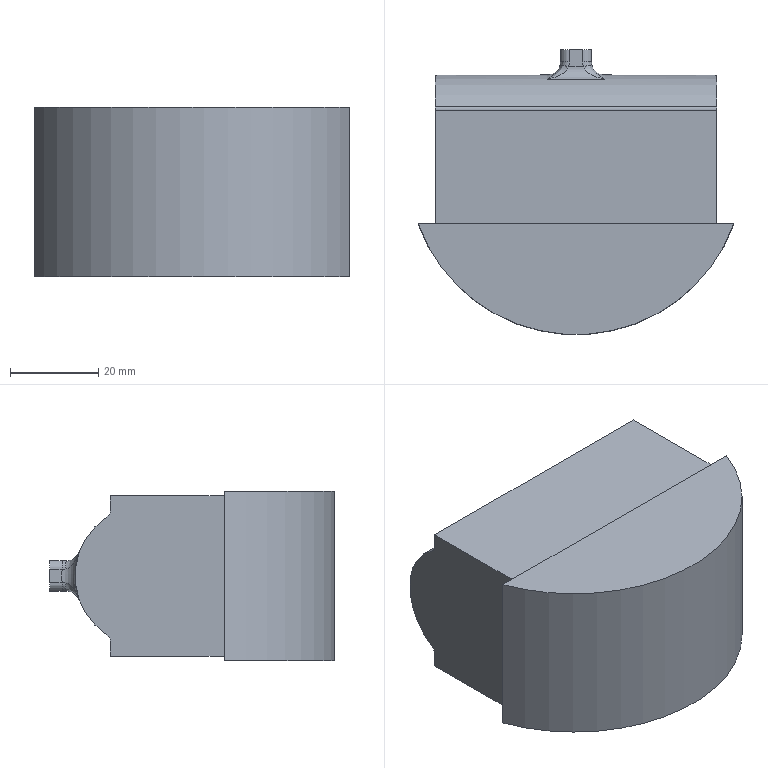NC program | NX | posted with a generic post | part box 71.627 x 64.667 x 38.42 mm
Lines 1 to 2470 of 24266, first 2159 of 2466 lines:
N10 G17 G21 G94 G90
(CAVITY_MILL , TOOL : D10)
N12 T00 M6
N14 G54
N16 G17 G0 G90 X23.164 Y-0.392 S2992 M3
N18 G43 Z10. H0
N20 Z0.2
N22 G94 G3 X14.3 Y0.708 Z-0.199 R-4.5 F1250.
N24 G1 Y-0.708 F2500.
N26 X14.41
N28 Y0.708
N30 X14.3
N32 Y5.208
N34 X8.926
N36 G2 X9.8 Y1.5 R8.3
N38 G1 Y-1.5
N40 G2 X8.926 Y-5.208 R8.3
N42 G1 X7.763 Y-4.627
N44 G2 X1.594 Y-8.499 R7.
N46 G1 X-1.599 Y-8.5
N48 G2 X-8.5 Y-1.5 R7.
N50 G1 Y1.5
N52 G2 X-1.5 Y8.5 R7.
N54 G1 X1.584
N56 G2 X8.5 Y1.5 R7.
N58 G1 Y-1.5
N60 G2 X7.763 Y-4.627 R7.
N62 G1 X8.926 Y-5.208
N64 X18.91
N66 Y5.208
N68 X14.3
N70 Y11.708
N72 X-14.3
N74 Y0.708
N76 X-14.41
N78 Y-0.708
N80 X-14.3
N82 Y0.708
N84 Y5.208
N86 X-18.91
N88 Y-5.208
N90 X-8.926
N92 G2 X-9.8 Y-1.5 R8.3
N94 G1 Y1.5
N96 G2 X-8.926 Y5.208 R8.3
N98 G1 X-14.3
N100 Y11.708
N102 X-25.41
N104 Y-11.708
N106 X25.41
N108 Y11.708
N110 X14.3
N112 Y18.208
N114 X-31.91
N116 Y-18.208
N118 X31.91
N120 Y18.208
N122 X14.3
N124 Y28.91
N126 Z0.001
N128 G0 Z0.3
N130 G1 X23.164 Y-0.392 F5000.
N132 G0 Z0.001
N134 G3 X14.3 Y0.708 Z-0.399 R-4.5 F1250.
N136 G1 Y-0.708 F2500.
N138 X14.41
N140 Y0.708
N142 X14.3
N144 Y5.208
N146 X8.926
N148 G2 X9.8 Y1.5 R8.3
N150 G1 Y-1.5
N152 G2 X8.926 Y-5.208 R8.3
N154 G1 X7.763 Y-4.627
N156 G2 X1.594 Y-8.499 R7.
N158 G1 X-1.599 Y-8.5
N160 G2 X-8.5 Y-1.5 R7.
N162 G1 Y1.5
N164 G2 X-1.5 Y8.5 R7.
N166 G1 X1.584
N168 G2 X8.5 Y1.5 R7.
N170 G1 Y-1.5
N172 G2 X7.763 Y-4.627 R7.
N174 G1 X8.926 Y-5.208
N176 X18.91
N178 Y5.208
N180 X14.3
N182 Y11.708
N184 X-14.3
N186 Y0.708
N188 X-14.41
N190 Y-0.708
N192 X-14.3
N194 Y0.708
N196 Y5.208
N198 X-18.91
N200 Y-5.208
N202 X-8.926
N204 G2 X-9.8 Y-1.5 R8.3
N206 G1 Y1.5
N208 G2 X-8.926 Y5.208 R8.3
N210 G1 X-14.3
N212 Y11.708
N214 X-25.41
N216 Y-11.708
N218 X25.41
N220 Y11.708
N222 X14.3
N224 Y18.208
N226 X-31.91
N228 Y-18.208
N230 X31.91
N232 Y18.208
N234 X14.3
N236 Y28.91
N238 Z-0.199
N240 G0 Z0.3
N242 G1 X23.164 Y-0.392 F5000.
N244 G0 Z-0.199
N246 G3 X14.3 Y0.708 Z-0.598 R-4.5 F1250.
N248 G1 Y-0.708 F2500.
N250 X14.41
N252 Y0.708
N254 X14.3
N256 Y5.208
N258 X8.926
N260 G2 X9.8 Y1.5 R8.3
N262 G1 Y-1.5
N264 G2 X8.926 Y-5.208 R8.3
N266 G1 X7.763 Y-4.627
N268 G2 X1.594 Y-8.499 R7.
N270 G1 X-1.599 Y-8.5
N272 G2 X-8.5 Y-1.5 R7.
N274 G1 Y1.5
N276 G2 X-1.5 Y8.5 R7.
N278 G1 X1.584
N280 G2 X8.5 Y1.5 R7.
N282 G1 Y-1.5
N284 G2 X7.763 Y-4.627 R7.
N286 G1 X8.926 Y-5.208
N288 X18.91
N290 Y5.208
N292 X14.3
N294 Y11.708
N296 X-14.3
N298 Y0.708
N300 X-14.41
N302 Y-0.708
N304 X-14.3
N306 Y0.708
N308 Y5.208
N310 X-18.91
N312 Y-5.208
N314 X-8.926
N316 G2 X-9.8 Y-1.5 R8.3
N318 G1 Y1.5
N320 G2 X-8.926 Y5.208 R8.3
N322 G1 X-14.3
N324 Y11.708
N326 X-25.41
N328 Y-11.708
N330 X25.41
N332 Y11.708
N334 X14.3
N336 Y18.208
N338 X-31.91
N340 Y-18.208
N342 X31.91
N344 Y18.208
N346 X14.3
N348 Y28.91
N350 Z-0.398
N352 G0 Z0.3
N354 G1 X23.164 Y-0.392 F5000.
N356 G0 Z-0.398
N358 G3 X14.3 Y0.708 Z-0.797 R-4.5 F1250.
N360 G1 Y-0.708 F2500.
N362 X14.41
N364 Y0.708
N366 X14.3
N368 Y5.208
N370 X8.926
N372 G2 X9.8 Y1.5 R8.3
N374 G1 Y-1.5
N376 G2 X8.926 Y-5.208 R8.3
N378 G1 X7.763 Y-4.627
N380 G2 X1.594 Y-8.499 R7.
N382 G1 X-1.599 Y-8.5
N384 G2 X-8.5 Y-1.5 R7.
N386 G1 Y1.5
N388 G2 X-1.5 Y8.5 R7.
N390 G1 X1.584
N392 G2 X8.5 Y1.5 R7.
N394 G1 Y-1.5
N396 G2 X7.763 Y-4.627 R7.
N398 G1 X8.926 Y-5.208
N400 X18.91
N402 Y5.208
N404 X14.3
N406 Y11.708
N408 X-14.3
N410 Y0.708
N412 X-14.41
N414 Y-0.708
N416 X-14.3
N418 Y0.708
N420 Y5.208
N422 X-18.91
N424 Y-5.208
N426 X-8.926
N428 G2 X-9.8 Y-1.5 R8.3
N430 G1 Y1.5
N432 G2 X-8.926 Y5.208 R8.3
N434 G1 X-14.3
N436 Y11.708
N438 X-25.41
N440 Y-11.708
N442 X25.41
N444 Y11.708
N446 X14.3
N448 Y18.208
N450 X-31.91
N452 Y-18.208
N454 X31.91
N456 Y18.208
N458 X14.3
N460 Y28.91
N462 Z-0.597
N464 G0 Z0.3
N466 G1 X23.164 Y-0.392 F5000.
N468 G0 Z-0.597
N470 G3 X14.3 Y0.708 Z-0.996 R-4.5 F1250.
N472 G1 Y-0.708 F2500.
N474 X14.41
N476 Y0.708
N478 X14.3
N480 Y5.208
N482 X8.926
N484 G2 X9.8 Y1.5 R8.3
N486 G1 Y-1.5
N488 G2 X8.926 Y-5.208 R8.3
N490 G1 X7.763 Y-4.627
N492 G2 X1.594 Y-8.499 R7.
N494 G1 X-1.599 Y-8.5
N496 G2 X-8.5 Y-1.5 R7.
N498 G1 Y1.5
N500 G2 X-1.5 Y8.5 R7.
N502 G1 X1.584
N504 G2 X8.5 Y1.5 R7.
N506 G1 Y-1.5
N508 G2 X7.763 Y-4.627 R7.
N510 G1 X8.926 Y-5.208
N512 X18.91
N514 Y5.208
N516 X14.3
N518 Y11.708
N520 X-14.3
N522 Y0.708
N524 X-14.41
N526 Y-0.708
N528 X-14.3
N530 Y0.708
N532 Y5.208
N534 X-18.91
N536 Y-5.208
N538 X-8.926
N540 G2 X-9.8 Y-1.5 R8.3
N542 G1 Y1.5
N544 G2 X-8.926 Y5.208 R8.3
N546 G1 X-14.3
N548 Y11.708
N550 X-25.41
N552 Y-11.708
N554 X25.41
N556 Y11.708
N558 X14.3
N560 Y18.208
N562 X-31.91
N564 Y-18.208
N566 X31.91
N568 Y18.208
N570 X14.3
N572 Y28.91
N574 Z-0.796
N576 G0 Z0.3
N578 G1 X23.164 Y-0.392 F5000.
N580 G0 Z-0.796
N582 G3 X14.3 Y0.708 Z-1.196 R-4.5 F1250.
N584 G1 Y-0.708 F2500.
N586 X14.41
N588 Y0.708
N590 X14.3
N592 Y5.208
N594 X8.926
N596 G2 X9.8 Y1.5 R8.3
N598 G1 Y-1.5
N600 G2 X8.926 Y-5.208 R8.3
N602 G1 X7.763 Y-4.627
N604 G2 X1.594 Y-8.499 R7.
N606 G1 X-1.599 Y-8.5
N608 G2 X-8.5 Y-1.5 R7.
N610 G1 Y1.5
N612 G2 X-1.5 Y8.5 R7.
N614 G1 X1.584
N616 G2 X8.5 Y1.5 R7.
N618 G1 Y-1.5
N620 G2 X7.763 Y-4.627 R7.
N622 G1 X8.926 Y-5.208
N624 X18.91
N626 Y5.208
N628 X14.3
N630 Y11.708
N632 X-14.3
N634 Y0.708
N636 X-14.41
N638 Y-0.708
N640 X-14.3
N642 Y0.708
N644 Y5.208
N646 X-18.91
N648 Y-5.208
N650 X-8.926
N652 G2 X-9.8 Y-1.5 R8.3
N654 G1 Y1.5
N656 G2 X-8.926 Y5.208 R8.3
N658 G1 X-14.3
N660 Y11.708
N662 X-25.41
N664 Y-11.708
N666 X25.41
N668 Y11.708
N670 X14.3
N672 Y18.208
N674 X-31.91
N676 Y-18.208
N678 X31.91
N680 Y18.208
N682 X14.3
N684 Y28.91
N686 Z-0.996
N688 G0 Z0.3
N690 G1 X23.164 Y-0.392 F5000.
N692 G0 Z-0.996
N694 G3 X14.3 Y0.708 Z-1.395 R-4.5 F1250.
N696 G1 Y-0.708 F2500.
N698 X14.41
N700 Y0.708
N702 X14.3
N704 Y5.208
N706 X8.926
N708 G2 X9.8 Y1.5 R8.3
N710 G1 Y-1.5
N712 G2 X8.926 Y-5.208 R8.3
N714 G1 X7.763 Y-4.627
N716 G2 X1.594 Y-8.499 R7.
N718 G1 X-1.599 Y-8.5
N720 G2 X-8.5 Y-1.5 R7.
N722 G1 Y1.5
N724 G2 X-1.5 Y8.5 R7.
N726 G1 X1.584
N728 G2 X8.5 Y1.5 R7.
N730 G1 Y-1.5
N732 G2 X7.763 Y-4.627 R7.
N734 G1 X8.926 Y-5.208
N736 X18.91
N738 Y5.208
N740 X14.3
N742 Y11.708
N744 X-14.3
N746 Y0.708
N748 X-14.41
N750 Y-0.708
N752 X-14.3
N754 Y0.708
N756 Y5.208
N758 X-18.91
N760 Y-5.208
N762 X-8.926
N764 G2 X-9.8 Y-1.5 R8.3
N766 G1 Y1.5
N768 G2 X-8.926 Y5.208 R8.3
N770 G1 X-14.3
N772 Y11.708
N774 X-25.41
N776 Y-11.708
N778 X25.41
N780 Y11.708
N782 X14.3
N784 Y18.208
N786 X-31.91
N788 Y-18.208
N790 X31.91
N792 Y18.208
N794 X14.3
N796 Y28.91
N798 Z-1.195
N800 G0 Z0.3
N802 G1 X23.164 Y-0.392 F5000.
N804 G0 Z-1.195
N806 G3 X14.3 Y0.708 Z-1.594 R-4.5 F1250.
N808 G1 Y-0.708 F2500.
N810 X14.41
N812 Y0.708
N814 X14.3
N816 Y5.208
N818 X8.926
N820 G2 X9.8 Y1.5 R8.3
N822 G1 Y-1.5
N824 G2 X8.926 Y-5.208 R8.3
N826 G1 X7.763 Y-4.627
N828 G2 X1.594 Y-8.499 R7.
N830 G1 X-1.599 Y-8.5
N832 G2 X-8.5 Y-1.5 R7.
N834 G1 Y1.5
N836 G2 X-1.5 Y8.5 R7.
N838 G1 X1.584
N840 G2 X8.5 Y1.5 R7.
N842 G1 Y-1.5
N844 G2 X7.763 Y-4.627 R7.
N846 G1 X8.926 Y-5.208
N848 X18.91
N850 Y5.208
N852 X14.3
N854 Y11.708
N856 X-14.3
N858 Y0.708
N860 X-14.41
N862 Y-0.708
N864 X-14.3
N866 Y0.708
N868 Y5.208
N870 X-18.91
N872 Y-5.208
N874 X-8.926
N876 G2 X-9.8 Y-1.5 R8.3
N878 G1 Y1.5
N880 G2 X-8.926 Y5.208 R8.3
N882 G1 X-14.3
N884 Y11.708
N886 X-25.41
N888 Y-11.708
N890 X25.41
N892 Y11.708
N894 X14.3
N896 Y18.208
N898 X-31.91
N900 Y-18.208
N902 X31.91
N904 Y18.208
N906 X14.3
N908 Y28.91
N910 Z-1.394
N912 G0 Z0.3
N914 G1 X23.164 Y-0.392 F5000.
N916 G0 Z-1.394
N918 G3 X14.3 Y0.708 Z-1.793 R-4.5 F1250.
N920 G1 Y-0.708 F2500.
N922 X14.41
N924 Y0.708
N926 X14.3
N928 Y5.208
N930 X8.926
N932 G2 X9.8 Y1.5 R8.3
N934 G1 Y-1.5
N936 G2 X8.926 Y-5.208 R8.3
N938 G1 X7.763 Y-4.627
N940 G2 X1.594 Y-8.499 R7.
N942 G1 X-1.599 Y-8.5
N944 G2 X-8.5 Y-1.5 R7.
N946 G1 Y1.5
N948 G2 X-1.5 Y8.5 R7.
N950 G1 X1.584
N952 G2 X8.5 Y1.5 R7.
N954 G1 Y-1.5
N956 G2 X7.763 Y-4.627 R7.
N958 G1 X8.926 Y-5.208
N960 X18.91
N962 Y5.208
N964 X14.3
N966 Y11.708
N968 X-14.3
N970 Y0.708
N972 X-14.41
N974 Y-0.708
N976 X-14.3
N978 Y0.708
N980 Y5.208
N982 X-18.91
N984 Y-5.208
N986 X-8.926
N988 G2 X-9.8 Y-1.5 R8.3
N990 G1 Y1.5
N992 G2 X-8.926 Y5.208 R8.3
N994 G1 X-14.3
N996 Y11.708
N998 X-25.41
N1000 Y-11.708
N1002 X25.41
N1004 Y11.708
N1006 X14.3
N1008 Y18.208
N1010 X-31.91
N1012 Y-18.208
N1014 X31.91
N1016 Y18.208
N1018 X14.3
N1020 Y28.91
N1022 Z-1.593
N1024 G0 Z0.3
N1026 G1 X23.164 Y-0.392 F5000.
N1028 G0 Z-1.593
N1030 G3 X14.3 Y0.708 Z-1.993 R-4.5 F1250.
N1032 G1 Y-0.708 F2500.
N1034 X14.41
N1036 Y0.708
N1038 X14.3
N1040 Y5.208
N1042 X8.926
N1044 G2 X9.8 Y1.5 R8.3
N1046 G1 Y-1.5
N1048 G2 X8.926 Y-5.208 R8.3
N1050 G1 X7.763 Y-4.627
N1052 G2 X1.594 Y-8.499 R7.
N1054 G1 X-1.599 Y-8.5
N1056 G2 X-8.5 Y-1.5 R7.
N1058 G1 Y1.5
N1060 G2 X-1.5 Y8.5 R7.
N1062 G1 X1.584
N1064 G2 X8.5 Y1.5 R7.
N1066 G1 Y-1.5
N1068 G2 X7.763 Y-4.627 R7.
N1070 G1 X8.926 Y-5.208
N1072 X18.91
N1074 Y5.208
N1076 X14.3
N1078 Y11.708
N1080 X-14.3
N1082 Y0.708
N1084 X-14.41
N1086 Y-0.708
N1088 X-14.3
N1090 Y0.708
N1092 Y5.208
N1094 X-18.91
N1096 Y-5.208
N1098 X-8.926
N1100 G2 X-9.8 Y-1.5 R8.3
N1102 G1 Y1.5
N1104 G2 X-8.926 Y5.208 R8.3
N1106 G1 X-14.3
N1108 Y11.708
N1110 X-25.41
N1112 Y-11.708
N1114 X25.41
N1116 Y11.708
N1118 X14.3
N1120 Y18.208
N1122 X-31.91
N1124 Y-18.208
N1126 X31.91
N1128 Y18.208
N1130 X14.3
N1132 Y28.91
N1134 Z-1.793
N1136 G0 Z0.3
N1138 G1 X23.164 Y-0.392 F5000.
N1140 G0 Z-1.793
N1142 G3 X14.3 Y0.708 Z-2.192 R-4.5 F1250.
N1144 G1 Y-0.708 F2500.
N1146 X14.41
N1148 Y0.708
N1150 X14.3
N1152 Y5.208
N1154 X8.926
N1156 G2 X9.8 Y1.5 R8.3
N1158 G1 Y-1.5
N1160 G2 X8.926 Y-5.208 R8.3
N1162 G1 X7.763 Y-4.627
N1164 G2 X1.594 Y-8.499 R7.
N1166 G1 X-1.599 Y-8.5
N1168 G2 X-8.5 Y-1.5 R7.
N1170 G1 Y1.5
N1172 G2 X-1.5 Y8.5 R7.
N1174 G1 X1.584
N1176 G2 X8.5 Y1.5 R7.
N1178 G1 Y-1.5
N1180 G2 X7.763 Y-4.627 R7.
N1182 G1 X8.926 Y-5.208
N1184 X18.91
N1186 Y5.208
N1188 X14.3
N1190 Y11.708
N1192 X-14.3
N1194 Y0.708
N1196 X-14.41
N1198 Y-0.708
N1200 X-14.3
N1202 Y0.708
N1204 Y5.208
N1206 X-18.91
N1208 Y-5.208
N1210 X-8.926
N1212 G2 X-9.8 Y-1.5 R8.3
N1214 G1 Y1.5
N1216 G2 X-8.926 Y5.208 R8.3
N1218 G1 X-14.3
N1220 Y11.708
N1222 X-25.41
N1224 Y-11.708
N1226 X25.41
N1228 Y11.708
N1230 X14.3
N1232 Y18.208
N1234 X-31.91
N1236 Y-18.208
N1238 X31.91
N1240 Y18.208
N1242 X14.3
N1244 Y28.91
N1246 Z-1.992
N1248 G0 Z0.3
N1250 G1 X23.164 Y-0.392 F5000.
N1252 G0 Z-1.992
N1254 G3 X14.3 Y0.708 Z-2.391 R-4.5 F1250.
N1256 G1 Y-0.708 F2500.
N1258 X14.41
N1260 Y0.708
N1262 X14.3
N1264 Y5.208
N1266 X8.926
N1268 G2 X9.8 Y1.5 R8.3
N1270 G1 Y-1.5
N1272 G2 X8.926 Y-5.208 R8.3
N1274 G1 X7.763 Y-4.627
N1276 G2 X1.594 Y-8.499 R7.
N1278 G1 X-1.599 Y-8.5
N1280 G2 X-8.5 Y-1.5 R7.
N1282 G1 Y1.5
N1284 G2 X-1.5 Y8.5 R7.
N1286 G1 X1.584
N1288 G2 X8.5 Y1.5 R7.
N1290 G1 Y-1.5
N1292 G2 X7.763 Y-4.627 R7.
N1294 G1 X8.926 Y-5.208
N1296 X18.91
N1298 Y5.208
N1300 X14.3
N1302 Y11.708
N1304 X-14.3
N1306 Y0.708
N1308 X-14.41
N1310 Y-0.708
N1312 X-14.3
N1314 Y0.708
N1316 Y5.208
N1318 X-18.91
N1320 Y-5.208
N1322 X-8.926
N1324 G2 X-9.8 Y-1.5 R8.3
N1326 G1 Y1.5
N1328 G2 X-8.926 Y5.208 R8.3
N1330 G1 X-14.3
N1332 Y11.708
N1334 X-25.41
N1336 Y-11.708
N1338 X25.41
N1340 Y11.708
N1342 X14.3
N1344 Y18.208
N1346 X-31.91
N1348 Y-18.208
N1350 X31.91
N1352 Y18.208
N1354 X14.3
N1356 Y28.91
N1358 Z-2.191
N1360 G0 Z0.3
N1362 G1 X23.164 Y-0.392 F5000.
N1364 G0 Z-2.191
N1366 G3 X14.3 Y0.708 Z-2.591 R-4.5 F1250.
N1368 G1 Y-0.708 F2500.
N1370 X14.41
N1372 Y0.708
N1374 X14.3
N1376 Y5.208
N1378 X8.926
N1380 G2 X9.8 Y1.5 R8.3
N1382 G1 Y-1.5
N1384 G2 X8.926 Y-5.208 R8.3
N1386 G1 X7.763 Y-4.627
N1388 G2 X1.594 Y-8.499 R7.
N1390 G1 X-1.599 Y-8.5
N1392 G2 X-8.5 Y-1.5 R7.
N1394 G1 Y1.5
N1396 G2 X-1.5 Y8.5 R7.
N1398 G1 X1.584
N1400 G2 X8.5 Y1.5 R7.
N1402 G1 Y-1.5
N1404 G2 X7.763 Y-4.627 R7.
N1406 G1 X8.926 Y-5.208
N1408 X18.91
N1410 Y5.208
N1412 X14.3
N1414 Y11.708
N1416 X-14.3
N1418 Y0.708
N1420 X-14.41
N1422 Y-0.708
N1424 X-14.3
N1426 Y0.708
N1428 Y5.208
N1430 X-18.91
N1432 Y-5.208
N1434 X-8.926
N1436 G2 X-9.8 Y-1.5 R8.3
N1438 G1 Y1.5
N1440 G2 X-8.926 Y5.208 R8.3
N1442 G1 X-14.3
N1444 Y11.708
N1446 X-25.41
N1448 Y-11.708
N1450 X25.41
N1452 Y11.708
N1454 X14.3
N1456 Y18.208
N1458 X-31.91
N1460 Y-18.208
N1462 X31.91
N1464 Y18.208
N1466 X14.3
N1468 Y28.91
N1470 Z-2.391
N1472 G0 Z0.3
N1474 G1 X23.164 Y-0.392 F5000.
N1476 G0 Z-2.391
N1478 G3 X14.3 Y0.708 Z-2.79 R-4.5 F1250.
N1480 G1 Y-0.708 F2500.
N1482 X14.41
N1484 Y0.708
N1486 X14.3
N1488 Y5.208
N1490 X8.926
N1492 G2 X9.8 Y1.5 R8.3
N1494 G1 Y-1.5
N1496 G2 X8.926 Y-5.208 R8.3
N1498 G1 X7.763 Y-4.627
N1500 G2 X1.594 Y-8.499 R7.
N1502 G1 X-1.599 Y-8.5
N1504 G2 X-8.5 Y-1.5 R7.
N1506 G1 Y1.5
N1508 G2 X-1.5 Y8.5 R7.
N1510 G1 X1.584
N1512 G2 X8.5 Y1.5 R7.
N1514 G1 Y-1.5
N1516 G2 X7.763 Y-4.627 R7.
N1518 G1 X8.926 Y-5.208
N1520 X18.91
N1522 Y5.208
N1524 X14.3
N1526 Y11.708
N1528 X-14.3
N1530 Y0.708
N1532 X-14.41
N1534 Y-0.708
N1536 X-14.3
N1538 Y0.708
N1540 Y5.208
N1542 X-18.91
N1544 Y-5.208
N1546 X-8.926
N1548 G2 X-9.8 Y-1.5 R8.3
N1550 G1 Y1.5
N1552 G2 X-8.926 Y5.208 R8.3
N1554 G1 X-14.3
N1556 Y11.708
N1558 X-25.41
N1560 Y-11.708
N1562 X25.41
N1564 Y11.708
N1566 X14.3
N1568 Y18.208
N1570 X-31.91
N1572 Y-18.208
N1574 X31.91
N1576 Y18.208
N1578 X14.3
N1580 Y28.91
N1582 Z-2.59
N1584 G0 Z0.3
N1586 G1 X23.184 Y-0.376 F5000.
N1588 G0 Z-2.59
N1590 G3 X14.318 Y0.708 Z-2.989 R-4.5 F1250.
N1592 G1 X14.321 Y-0.708 F2500.
N1594 X14.41
N1596 Y0.708
N1598 X14.318
N1600 Y5.208
N1602 X8.938
N1604 G2 X9.79 Y1.997 R8.239
N1606 G1 X9.815 Y1.577
N1608 X9.817 Y1.503
N1610 X9.822 Y-1.498
N1612 X9.819 Y-1.592
N1614 X9.79 Y-2.006
N1616 G2 X8.935 Y-5.208 R8.288
N1618 G1 X7.771 Y-4.628
N1620 G2 X1.858 Y-8.491 R6.988
N1622 X1.594 Y-8.499 R7.
N1624 G1 X-1.599 Y-8.5
N1626 G2 X-1.886 Y-8.489 R7.
N1628 X-8.517 Y-1.5 R7.012
N1630 G1 X-8.522 Y1.5
N1632 X-8.496 Y1.922
N1634 G2 X-1.939 Y8.486 R6.994
N1636 X-1.5 Y8.5 R7.
N1638 G1 X1.584
N1640 G2 X4.913 Y7.612 R7.
N1642 X8.492 Y1.922 R6.939
N1644 G1 X8.517 Y1.5
N1646 X8.522 Y-1.5
N1648 X8.492 Y-1.922
N1650 G2 X7.771 Y-4.628 R6.988
N1652 G1 X8.935 Y-5.208
N1654 X18.91
N1656 Y5.208
N1658 X14.318
N1660 Y11.708
N1662 X-14.321
N1664 Y0.708
N1666 X-14.41
N1668 Y-0.708
N1670 X-14.318
N1672 X-14.321 Y0.708
N1674 Y5.208
N1676 X-18.91
N1678 Y-5.208
N1680 X-8.938
N1682 G2 X-9.817 Y-1.503 R8.312
N1684 G1 X-9.822 Y1.498
N1686 X-9.82 Y1.582
N1688 X-9.793 Y2.002
N1690 G2 X-8.936 Y5.208 R8.294
N1692 G1 X-14.321
N1694 Y11.708
N1696 X-25.41
N1698 Y-11.708
N1700 X25.41
N1702 Y11.708
N1704 X14.318
N1706 Y18.208
N1708 X-31.91
N1710 Y-18.208
N1712 X31.91
N1714 Y18.208
N1716 X14.318
N1718 Y28.91
N1720 Z-2.789
N1722 G0 Z0.3
N1724 G1 X23.211 Y-0.382 F5000.
N1726 G0 Z-2.789
N1728 G3 X14.346 Y0.708 Z-3.188 R-4.5 F1250.
N1730 G1 X14.348 Y-0.708 F2500.
N1732 X14.41
N1734 Y0.708
N1736 X14.346
N1738 Y5.208
N1740 X8.963
N1742 G2 X9.81 Y2.008 R8.182
N1744 G1 X9.841 Y1.602
N1746 X9.845 Y1.502
N1748 X9.849 Y-1.499
N1750 X9.844 Y-1.613
N1752 X9.809 Y-2.017
N1754 G2 X8.955 Y-5.208 R8.282
N1756 G1 X7.792 Y-4.628
N1758 G2 X1.88 Y-8.49 R6.982
N1760 X1.594 Y-8.499 R7.
N1762 G1 X-1.599 Y-8.5
N1764 G2 X-1.877 Y-8.49 R7.
N1766 X-8.517 Y-1.922 R6.992
N1768 G1 X-8.545 Y-1.501
N1770 X-8.549 Y1.501
N1772 X-8.514 Y1.922
N1774 G2 X-1.909 Y8.488 R6.984
N1776 X-1.587 Y8.499 R7.
N1778 G1 X1.584 Y8.5
N1780 G2 X4.913 Y7.612 R7.
N1782 X8.512 Y1.922 R6.882
N1784 G1 X8.545 Y1.501
N1786 X8.549 Y-1.501
N1788 X8.512 Y-1.922
N1790 G2 X7.792 Y-4.628 R6.982
N1792 G1 X8.955 Y-5.208
N1794 X18.91
N1796 Y5.208
N1798 X14.346
N1800 Y11.708
N1802 X-14.348
N1804 Y0.708
N1806 X-14.41
N1808 Y-0.708
N1810 X-14.346
N1812 X-14.348 Y0.708
N1814 Y5.208
N1816 X-18.91
N1818 Y-5.208
N1820 X-8.958
N1822 G2 X-9.815 Y-2.004 R8.292
N1824 G1 X-9.842 Y-1.587
N1826 X-9.845 Y-1.502
N1828 X-9.849 Y1.499
N1830 X-9.844 Y1.606
N1832 X-9.811 Y2.014
N1834 G2 X-8.957 Y5.208 R8.284
N1836 G1 X-14.348
N1838 Y11.708
N1840 X-25.41
N1842 Y-11.708
N1844 X25.41
N1846 Y11.708
N1848 X14.346
N1850 Y18.208
N1852 X-31.91
N1854 Y-18.208
N1856 X31.91
N1858 Y18.208
N1860 X14.346
N1862 Y28.91
N1864 Z-2.988
N1866 G0 Z0.3
N1868 G1 X23.238 Y-0.388 F5000.
N1870 G0 Z-2.988
N1872 G3 X14.374 Y0.708 Z-3.388 R-4.5 F1250.
N1874 G1 X14.375 Y-0.708 F2500.
N1876 X14.41
N1878 Y0.708
N1880 X14.374
N1882 Y5.208
N1884 X8.983
N1886 G2 X9.84 Y2.008 R8.288
N1888 G1 X9.87 Y1.595
N1890 X9.874 Y1.502
N1892 X9.875 Y-1.501
N1894 X9.871 Y-1.605
N1896 X9.838 Y-2.013
N1898 G2 X8.982 Y-5.208 R8.29
N1900 G1 X7.819 Y-4.627
N1902 G2 X1.858 Y-8.491 R6.99
N1904 X1.594 Y-8.499 R7.
N1906 G1 X-1.599 Y-8.5
N1908 G2 X-1.877 Y-8.49 R7.
N1910 X-8.543 Y-1.922 R6.995
N1912 G1 X-8.574 Y-1.501
N1914 X-8.575 Y1.501
N1916 X-8.541 Y1.922
N1918 G2 X-1.909 Y8.488 R6.989
N1920 X-1.587 Y8.499 R7.
N1922 G1 X1.584 Y8.5
N1924 G2 X2.099 Y8.474 R7.
N1926 X8.543 Y1.922 R6.988
N1928 G1 X8.574 Y1.501
N1930 X8.575 Y-1.501
N1932 X8.541 Y-1.922
N1934 G2 X7.819 Y-4.627 R6.99
N1936 G1 X8.982 Y-5.208
N1938 X18.91
N1940 Y5.208
N1942 X14.374
N1944 Y11.708
N1946 X-14.375
N1948 Y0.708
N1950 X-14.41
N1952 Y-0.708
N1954 X-14.374
N1956 X-14.375 Y0.708
N1958 Y5.208
N1960 X-18.91
N1962 Y-5.208
N1964 X-8.982
N1966 G2 X-9.84 Y-2.009 R8.295
N1968 G1 X-9.87 Y-1.595
N1970 X-9.874 Y-1.502
N1972 X-9.875 Y1.501
N1974 X-9.871 Y1.605
N1976 X-9.838 Y2.013
N1978 G2 X-8.982 Y5.208 R8.289
N1980 G1 X-14.375
N1982 Y11.708
N1984 X-25.41
N1986 Y-11.708
N1988 X25.41
N1990 Y11.708
N1992 X14.374
N1994 Y18.208
N1996 X-31.91
N1998 Y-18.208
N2000 X31.91
N2002 Y18.208
N2004 X14.374
N2006 Y28.91
N2008 Z-3.188
N2010 G0 Z0.3
N2012 G1 X17.435 Y8.208 F5000.
N2014 G0 Z-3.188
N2016 G3 X9.023 Y5.208 Z-3.587 R-4.5 F1250.
N2018 G2 X9.911 Y1.525 R8.327 F2500.
N2020 G1 X9.92 Y1.191
N2022 X9.921 Y1.153
N2024 Y-1.153
N2026 X9.92 Y-1.191
N2028 X9.911 Y-1.525
N2030 G2 X9.023 Y-5.208 R8.332
N2032 G1 X7.861 Y-4.623
N2034 G2 X1.858 Y-8.491 R7.032
N2036 X1.594 Y-8.499 R7.
N2038 G1 X-1.599 Y-8.5
N2040 G2 X-1.877 Y-8.49 R7.
N2042 X-8.611 Y-1.502 R7.029
N2044 G1 X-8.621 Y-1.153
N2046 Y1.153
N2048 X-8.611 Y1.502
N2050 G2 X-1.909 Y8.488 R7.027
N2052 X-1.587 Y8.499 R7.
N2054 G1 X1.584 Y8.5
N2056 G2 X2.099 Y8.474 R7.
N2058 X8.611 Y1.502 R7.027
N2060 G1 X8.621 Y1.153
N2062 Y-1.153
N2064 X8.611 Y-1.502
N2066 G2 X7.861 Y-4.623 R7.032
N2068 G1 X9.023 Y-5.208
N2070 X18.91
N2072 Y5.208
N2074 X9.023
N2076 Y11.708
N2078 X-9.024
N2080 Y5.208
N2082 X-18.91
N2084 Y-5.208
N2086 X-9.023
N2088 G2 X-9.911 Y-1.524 R8.329
N2090 G1 X-9.92 Y-1.191
N2092 X-9.921 Y-1.153
N2094 Y1.153
N2096 X-9.92 Y1.191
N2098 X-9.911 Y1.524
N2100 G2 X-9.024 Y5.208 R8.327
N2102 G1 Y11.708
N2104 X-25.41
N2106 Y-11.708
N2108 X25.41
N2110 Y11.708
N2112 X9.023
N2114 Y18.208
N2116 X-31.91
N2118 Y-18.208
N2120 X31.91
N2122 Y18.208
N2124 X9.023
N2126 Y28.91
N2128 Z-3.387
N2130 G0 Z0.3
N2132 G1 X17.5 Y8.202 F5000.
N2134 G0 Z-3.387
N2136 G3 X9.085 Y5.208 Z-3.786 R-4.5 F1250.
N2138 G2 X9.968 Y1.547 R8.308 F2500.
N2140 G1 X9.98 Y1.198
N2142 X9.981 Y1.153
N2144 Y-1.153
N2146 X9.98 Y-1.197
N2148 X9.968 Y-1.546
N2150 G2 X9.085 Y-5.208 R8.318
N2152 G1 X7.921 Y-4.624
N2154 G2 X1.858 Y-8.491 R7.018
N2156 X1.594 Y-8.499 R7.
N2158 G1 X-1.599 Y-8.5
N2160 G2 X-1.877 Y-8.49 R7.
N2162 X-8.576 Y-2.691 R7.063
N2164 X-8.576 Y2.691 R28.187
N2166 X-1.909 Y8.488 R7.057
N2168 X-1.587 Y8.499 R7.
N2170 G1 X1.584 Y8.5
N2172 G2 X2.099 Y8.474 R7.
N2174 X8.652 Y1.922 R7.008
N2176 G1 X8.669 Y1.503
N2178 X8.681 Y1.153
N2180 Y-1.153
N2182 X8.669 Y-1.503
N2184 X8.653 Y-1.922
N2186 G2 X7.921 Y-4.624 R7.018
N2188 G1 X9.085 Y-5.208
N2190 X18.91
N2192 Y5.208
N2194 X9.085
N2196 Y11.708
N2198 X-9.089
N2200 Y5.208
N2202 X-18.91
N2204 Y-5.208
N2206 X-9.088
N2208 G2 X-9.855 Y-2.923 R8.363
N2210 G1 X-9.87 Y-2.815
N2212 G2 X-9.87 Y2.815 R29.488
N2214 G1 X-9.855 Y2.922
N2216 G2 X-9.089 Y5.208 R8.357
N2218 G1 Y11.708
N2220 X-25.41
N2222 Y-11.708
N2224 X25.41
N2226 Y11.708
N2228 X9.085
N2230 Y18.208
N2232 X-31.91
N2234 Y-18.208
N2236 X31.91
N2238 Y18.208
N2240 X9.085
N2242 Y28.91
N2244 Z-3.586
N2246 G0 Z0.3
N2248 G1 X17.592 Y8.186 F5000.
N2250 G0 Z-3.586
N2252 G3 X9.171 Y5.208 Z-3.986 R-4.5 F1250.
N2254 G2 X10.035 Y1.932 R8.306 F2500.
N2256 X10.038 Y-1.989 R37.796
N2258 X9.182 Y-5.208 R8.22
N2260 G1 X8.019 Y-4.626
N2262 G2 X4.621 Y-7.861 R6.92
N2264 G1 X4.351 Y-7.974
N2266 G2 X1.714 Y-8.501 R6.854
N2268 G1 X1.42
N2270 Y-8.5
N2272 X-1.372
N2274 Y-8.501
N2276 X-1.584
N2278 Y-8.5
N2280 X-1.599
N2282 X-1.657 Y-8.498
N2284 G2 X-8.737 Y-1.922 R7.008
N2286 G1 X-8.754 Y-1.504
N2288 G2 X-8.74 Y1.922 R36.496
N2290 X-4.621 Y7.861 R6.92
N2292 X-1.679 Y8.498 R6.882
N2294 G1 X-1.61 Y8.499
N2296 Y8.501
N2298 X-1.372
N2300 Y8.5
N2302 X1.42
N2304 Y8.501
N2306 X1.741
N2308 G2 X8.737 Y1.864 R7.006
N2310 X8.74 Y-1.922 R36.496
N2312 X8.019 Y-4.626 R6.92
N2314 G1 X9.182 Y-5.208
N2316 X18.91
N2318 Y5.208
N2320 X9.171
N2322 Y11.708
N2324 X-9.182
N2326 Y5.208
N2328 X-18.91
N2330 Y-5.208
N2332 X-9.176
N2334 G2 X-10.053 Y-1.559 R8.308
N2336 X-10.038 Y1.989 R37.796
N2338 X-9.182 Y5.208 R8.22
N2340 G1 Y11.708
N2342 X-25.41
N2344 Y-11.708
N2346 X25.41
N2348 Y11.708
N2350 X9.171
N2352 Y18.208
N2354 X-31.91
N2356 Y-18.208
N2358 X31.91
N2360 Y18.208
N2362 X9.171
N2364 Y28.91
N2366 Z-3.786
N2368 G0 Z0.3
N2370 G1 X17.734 Y8.157 F5000.
N2372 G0 Z-3.786
N2374 G3 X9.303 Y5.208 Z-4.185 R-4.5 F1250.
N2376 G2 X10.133 Y1.981 R8.054 F2500.
N2378 X10.133 Y-1.982 R41.78
N2380 X9.303 Y-5.208 R8.141
N2382 G1 X8.137 Y-4.633
N2384 G2 X4.621 Y-7.927 R6.841
N2386 G1 X4.447 Y-7.998
N2388 G2 X1.8 Y-8.514 R7.045
N2390 G1 X-1.658
N2392 G2 X-6.751 Y-6.536 R7.262
N2394 X-8.834 Y-1.922 R6.833
N2396 X-8.834 Y1.937 R40.464
N2398 X-5.006 Y7.74 R6.815
N2400 G1 X-4.861 Y7.811
N2402 G2 X-1.807 Y8.514 R6.984
N2404 G1 X1.672
N2406 G2 X7.942 Y4.998 R7.088
N2408 X8.834 Y1.922 R6.754
N2410 X8.834 Y-1.922 R40.48
N2412 X8.137 Y-4.633 R6.841
N2414 G1 X9.303 Y-5.208
N2416 X18.91
N2418 Y5.208
N2420 X9.303
N2422 Y11.708
N2424 X-9.301
N2426 Y5.208
N2428 X-18.91
N2430 Y-5.208
N2432 X-9.305
N2434 G2 X-10.133 Y-1.982 R8.133
N2436 X-10.132 Y2. R41.764
N2438 X-9.301 Y5.208 R8.115
N2440 G1 Y11.708
N2442 X-25.41
N2444 Y-11.708
N2446 X25.41
N2448 Y11.708
N2450 X9.303
N2452 Y18.208
N2454 X-31.91
N2456 Y-18.208
N2458 X31.91
N2460 Y18.208
N2462 X9.303
N2464 Y28.91
N2466 Z-3.985
N2468 G0 Z0.3
N2470 G1 X17.914 Y8.036 F5000.
N2472 G0 Z-3.985
N2474 G3 X9.442 Y5.208 Z-4.384 R-4.5 F1250.
N2476 G2 X10.245 Y1.984 R8.3 F2500.
N2478 X10.245 Y-1.981 R37.26
N2480 X9.443 Y-5.208 R8.115
N2482 G1 X8.272 Y-4.642
N2484 G2 X3.851 Y-8.272 R6.815
N2486 X1.831 Y-8.54 R6.997
N2488 G1 X-1.785
N2490 G2 X-7.603 Y-5.767 R7.192
N2492 X-8.947 Y-1.922 R7.031
N2494 X-8.947 Y1.922 R35.931
N2496 X-3.851 Y8.272 R6.815
N2498 X-1.895 Y8.54 R6.893
N2500 G1 X1.804
N2502 G2 X7.6 Y5.767 R7.19
N2504 X8.947 Y1.922 R7.
N2506 X8.947 Y-1.922 R35.96
N2508 X8.272 Y-4.642 R6.815
N2510 G1 X9.443 Y-5.208
N2512 X18.91
N2514 Y5.208
N2516 X9.442
N2518 Y11.708
N2520 X-9.443
N2522 Y5.208
N2524 X-18.91
N2526 Y-5.208
N2528 X-9.443
N2530 G2 X-10.245 Y-1.985 R8.331
N2532 X-10.245 Y1.981 R37.231
N2534 X-9.443 Y5.208 R8.115
N2536 G1 Y11.708
N2538 X-25.41
N2540 Y-11.708
N2542 X25.41
N2544 Y11.708
N2546 X9.442
N2548 Y18.208
N2550 X-31.91
N2552 Y-18.208
N2554 X31.91
N2556 Y18.208
N2558 X9.442
N2560 Y28.91
N2562 Z-4.184
N2564 G0 Z0.3
N2566 G1 X18.126 Y7.911 F5000.
N2568 G0 Z-4.184
N2570 G3 X9.613 Y5.208 Z-4.583 R-4.5 F1250.
N2572 G2 X10.282 Y2.849 R7.967 F2500.
N2574 X10.306 Y-2.677 R26.083
N2576 X9.609 Y-5.208 R7.908
N2578 G1 X8.431 Y-4.659
N2580 G2 X5.011 Y-7.96 R6.608
N2582 G1 X4.741 Y-8.074
N2584 G2 X2.06 Y-8.58 R7.047
N2586 G1 X-2.06
N2588 G2 X-7.147 Y-6.536 R7.282
N2590 X-8.992 Y-2.691 R6.667
N2592 X-9.011 Y2.559 R24.783
N2594 X-5.02 Y7.956 R6.59
N2596 G1 X-4.741 Y8.074
N2598 G2 X-1.964 Y8.58 R7.193
N2600 G1 X2.06
N2602 G2 X7.147 Y6.536 R7.267
N2604 X8.992 Y2.691 R6.667
N2606 X9.013 Y-2.545 R24.783
N2608 X8.431 Y-4.659 R6.608
N2610 G1 X9.609 Y-5.208
N2612 X18.91
N2614 Y5.208
N2616 X9.613
N2618 Y11.708
N2620 X-9.612
N2622 Y5.208
N2624 X-18.91
N2626 Y-5.208
N2628 X-9.613
N2630 G2 X-10.282 Y-2.849 R7.967
N2632 X-10.304 Y2.692 R26.083
N2634 X-9.612 Y5.208 R7.89
N2636 G1 Y11.708
N2638 X-25.41
N2640 Y-11.708
N2642 X25.41
N2644 Y11.708
N2646 X9.613
N2648 Y18.208
N2650 X-31.91
N2652 Y-18.208
N2654 X31.91
N2656 Y18.208
N2658 X9.613
N2660 Y28.91
N2662 Z-4.383
N2664 G0 Z0.3
N2666 G1 X18.351 Y7.804 F5000.
N2668 G0 Z-4.383
N2670 G3 X9.805 Y5.208 Z-4.783 R-4.5 F1250.
N2672 G2 X10.442 Y2.84 R7.923 F2500.
N2674 X10.445 Y-2.841 R23.274
N2676 X9.801 Y-5.208 R7.901
N2678 G1 X8.614 Y-4.675
N2680 G2 X3.851 Y-8.453 R6.601
N2682 X2.252 Y-8.634 R6.14
N2684 G1 X-2.252
N2686 G2 X-6.162 Y-7.535 R7.46
N2688 X-9.151 Y-2.691 R6.541
N2690 X-9.133 Y2.851 R21.868
N2692 X-4.197 Y8.368 R6.559
N2694 G1 X-3.851 Y8.453
N2696 G2 X-2.252 Y8.634 R7.951
N2698 G1 X2.108
N2700 G2 X6.932 Y6.969 R7.311
N2702 X9.151 Y2.691 R6.623
N2704 X9.154 Y-2.691 R21.974
N2706 X8.614 Y-4.675 R6.601
N2708 G1 X9.801 Y-5.208
N2710 X18.91
N2712 Y5.208
N2714 X9.805
N2716 Y11.708
N2718 X-9.804
N2720 Y5.208
N2722 X-18.91
N2724 Y-5.208
N2726 X-9.808
N2728 G2 X-10.442 Y-2.839 R7.841
N2730 X-10.422 Y3.019 R23.168
N2732 X-9.804 Y5.208 R7.859
N2734 G1 Y11.708
N2736 X-25.41
N2738 Y-11.708
N2740 X25.41
N2742 Y11.708
N2744 X9.805
N2746 Y18.208
N2748 X-31.91
N2750 Y-18.208
N2752 X31.91
N2754 Y18.208
N2756 X9.805
N2758 Y28.91
N2760 Z-4.583
N2762 G0 Z0.3
N2764 G1 X18.641 Y7.61 F5000.
N2766 G0 Z-4.583
N2768 G3 X10.038 Y5.208 Z-4.982 R-4.5 F1250.
N2770 G2 X10.469 Y3.784 R7.321 F2500.
N2772 X10.524 Y-3.476 R19.751
N2774 X10.021 Y-5.208 R7.695
N2776 G1 X8.824 Y-4.701
N2778 G2 X5.392 Y-8.115 R6.395
N2780 X2.311 Y-8.703 R7.439
N2782 G1 X-2.472
N2784 G2 X-9.013 Y-4.229 R6.752
N2786 X-9.013 Y4.229 R17.194
N2788 X-3.081 Y8.682 R6.693
N2790 G1 X-2.311 Y8.703
N2792 X2.59
N2794 G2 X7.645 Y6.536 R6.977
N2796 X9.193 Y3.536 R6.021
N2798 X9.243 Y-3.255 R18.451
N2800 X8.824 Y-4.701 R6.395
N2802 G1 X10.021 Y-5.208
N2804 X18.91
N2806 Y5.208
N2808 X10.038
N2810 Y11.708
N2812 X-10.023
N2814 Y5.208
N2816 X-18.91
N2818 Y-5.208
N2820 X-10.021
N2822 G2 X-10.237 Y-4.667 R8.052
N2824 G1 X-10.273 Y-4.549
N2826 G2 X-10.273 Y4.549 R18.494
N2828 G1 X-10.239 Y4.662
N2830 G2 X-10.023 Y5.208 R7.993
N2832 G1 Y11.708
N2834 X-25.41
N2836 Y-11.708
N2838 X25.41
N2840 Y11.708
N2842 X10.038
N2844 Y18.208
N2846 X-31.91
N2848 Y-18.208
N2850 X31.91
N2852 Y18.208
N2854 X10.038
N2856 Y28.91
N2858 Z-4.782
N2860 G0 Z0.3
N2862 G1 X18.915 Y7.474 F5000.
N2864 G0 Z-4.782
N2866 G3 X10.276 Y5.208 Z-5.181 R-4.5 F1250.
N2868 G2 X10.642 Y4.013 R7.563 F2500.
N2870 X10.705 Y-3.704 R18.835
N2872 X10.271 Y-5.208 R7.699
N2874 G1 X9.065 Y-4.722
N2876 G2 X4.57 Y-8.565 R6.399
N2878 X2.609 Y-8.789 R8.713
N2880 G1 X-2.973
N2882 G2 X-9.388 Y-3.62 R6.565
N2884 X-9.241 Y4.229 R16.991
N2886 X-3.081 Y8.783 R6.562
N2888 G1 X-2.723 Y8.789
N2890 X2.859
N2892 G2 X6.826 Y7.546 R6.953
N2894 X9.372 Y3.736 R6.263
N2896 X9.428 Y-3.46 R17.535
N2898 X9.065 Y-4.722 R6.399
N2900 G1 X10.271 Y-5.208
N2902 X18.91
N2904 Y5.208
N2906 X10.276
N2908 Y11.708
N2910 X-10.264
N2912 Y5.208
N2914 X-18.91
N2916 Y-5.208
N2918 X-10.25
N2920 G2 X-10.658 Y-3.897 R7.865
N2922 X-10.5 Y4.553 R18.291
N2924 X-10.264 Y5.208 R7.862
N2926 G1 Y11.708
N2928 X-25.41
N2930 Y-11.708
N2932 X25.41
N2934 Y11.708
N2936 X10.276
N2938 Y18.208
N2940 X-31.91
N2942 Y-18.208
N2944 X31.91
N2946 Y18.208
N2948 X10.276
N2950 Y28.91
N2952 Z-4.981
N2954 G0 Z0.3
N2956 G1 X19.219 Y7.292 F5000.
N2958 G0 Z-4.981
N2960 G3 X10.534 Y5.208 Z-5.38 R-4.5 F1250.
N2962 G2 X10.737 Y4.585 R7.612 F2500.
N2964 X10.942 Y-3.758 R16.425
N2966 G1 X10.825 Y-4.258
N2968 G2 X10.536 Y-5.208 R7.625
N2970 G1 X9.32 Y-4.749
N2972 G2 X4.467 Y-8.755 R6.325
N2974 X2.847 Y-8.893 R9.605
N2976 G1 X-2.908
N2978 G2 X-4.595 Y-8.732 R8.964
N2980 X-9.487 Y-4.229 R6.312
N2982 X-9.677 Y3.46 R15.125
N2984 G1 X-9.562 Y3.95
N2986 G2 X-3.864 Y8.846 R6.368
N2988 X-2.694 Y8.893 R14.827
N2990 G1 X2.897
N2992 G2 X4.571 Y8.737 R9.077
N2994 X9.487 Y4.229 R6.312
N2996 X9.677 Y-3.46 R15.125
N2998 G1 X9.559 Y-3.962
N3000 G2 X9.32 Y-4.749 R6.325
N3002 G1 X10.536 Y-5.208
N3004 X18.91
N3006 Y5.208
N3008 X10.534
N3010 Y11.708
N3012 X-10.535
N3014 Y5.208
N3016 X-18.91
N3018 Y-5.208
N3020 X-10.534
N3022 G2 X-10.737 Y-4.585 R7.612
N3024 X-10.942 Y3.758 R16.425
N3026 G1 X-10.828 Y4.246
N3028 G2 X-10.535 Y5.208 R7.668
N3030 G1 Y11.708
N3032 X-25.41
N3034 Y-11.708
N3036 X25.41
N3038 Y11.708
N3040 X10.534
N3042 Y18.208
N3044 X-31.91
N3046 Y-18.208
N3048 X31.91
N3050 Y18.208
N3052 X10.534
N3054 Y28.91
N3056 Z-5.18
N3058 G0 Z0.3
N3060 G1 X19.613 Y6.917 F5000.
N3062 G0 Z-5.18
N3064 G3 X10.847 Y5.208 Z-5.58 R-4.5 F1250.
N3066 G1 X11.031 Y4.644 F2500.
N3068 G2 X10.843 Y-5.208 R14.289
N3070 G1 X9.631 Y-4.736
N3072 G2 X9.178 Y-5.767 R12.989
N3074 X3.851 Y-9.012 R6.497
N3076 G1 X3.32 Y-9.017
N3078 X-3.081
N3080 X-3.141 Y-9.019
N3082 G2 X-9.548 Y-4.998 R6.538
N3084 G1 X-9.799 Y-4.229
N3086 G2 X-9.178 Y5.767 R12.989
N3088 X-3.851 Y9.012 R6.482
N3090 G1 X-3.32 Y9.017
N3092 X3.081
N3094 X3.141 Y9.019
N3096 G2 X9.548 Y4.998 R6.538
N3098 G1 X9.799 Y4.229
N3100 G2 X9.631 Y-4.736 R12.989
N3102 G1 X10.843 Y-5.208
N3104 X18.91
N3106 Y5.208
N3108 X10.847
N3110 Y11.708
N3112 X-10.843
N3114 Y5.208
N3116 X-18.91
N3118 Y-5.208
N3120 X-10.847
N3122 X-11.031 Y-4.644
N3124 G2 X-10.843 Y5.208 R14.289
N3126 G1 Y11.708
N3128 X-25.41
N3130 Y-11.708
N3132 X25.41
N3134 Y11.708
N3136 X10.847
N3138 Y18.208
N3140 X-31.91
N3142 Y-18.208
N3144 X31.91
N3146 Y18.208
N3148 X10.847
N3150 Y28.91
N3152 Z-5.38
N3154 G0 Z0.3
N3156 G1 X4.832 Y-14.807 F5000.
N3158 G0 Z-5.38
N3160 G3 X-4.032 Y-13.708 Z-5.779 R-4.5 F1250.
N3162 G1 X0.468
N3164 X27.41 F2500.
N3166 Y-10.463
N3168 X11.612
N3170 G2 X3.928 Y-13.664 R10.82
N3172 G1 X-3.9
N3174 G2 X-11.619 Y-10.463 R10.906
N3176 G1 X-27.41
N3178 Y-13.708
N3180 X0.468
N3182 Y-18.208
N3184 X31.91
N3186 Y-5.963
N3188 X9.425
N3190 G2 X3.928 Y-9.164 R6.32
N3192 G1 X-3.9
N3194 G2 X-9.447 Y-5.963 R6.406
N3196 G1 X-31.91
N3198 Y-18.208
N3200 X0.468
N3202 Y-28.91
N3204 Z-5.579
N3206 G0 Z0.3
N3208 G1 X10.351 Y-14.807 F5000.
N3210 G0 Z-5.579
N3212 G3 X1.488 Y-13.708 Z-5.978 R-4.5 F1250.
N3214 G1 X5.988
N3216 X27.41 F2500.
N3218 Y-12.193
N3220 X10.064
N3222 G2 X5.988 Y-13.708 R11.025
N3224 G1 Y-18.208
N3226 X31.91
N3228 Y-7.693
N3230 X8.599
N3232 G2 X4.241 Y-9.344 R6.525
N3234 G1 X3.081 Y-9.34
N3236 X-4.085
N3238 G2 X-5.26 Y-9.261 R6.693
N3240 G1 X-5.954 Y-13.708
N3242 G2 X-10.074 Y-12.193 R11.193
N3244 G1 X-27.41
N3246 Y-13.708
N3248 X-5.954
N3250 X-5.26 Y-9.261
N3252 G2 X-8.626 Y-7.693 R6.693
N3254 G1 X-31.91
N3256 Y-18.208
N3258 X5.988
N3260 Y-28.91
N3262 Z-5.778
N3264 G0 Z0.3
N3266 G1 X11.849 Y-14.807 F5000.
N3268 G0 Z-5.778
N3270 G3 X2.985 Y-13.708 Z-6.178 R-4.5 F1250.
N3272 G1 X7.485
N3274 X27.41 F2500.
N3276 Y-13.174
N3278 X9.026
N3280 G2 X7.485 Y-13.708 R10.565
N3282 G1 Y-18.208
N3284 X31.91
N3286 Y-8.674
N3288 X7.953
N3290 G2 X4.811 Y-9.552 R6.065
N3292 G1 X-4.797
N3294 G2 X-6.351 Y-9.353 R6.171
N3296 G1 X-7.484 Y-13.708
N3298 G2 X-9.034 Y-13.174 R10.671
N3300 G1 X-27.41
N3302 Y-13.708
N3304 X-7.484
N3306 X-6.351 Y-9.353
N3308 G2 X-7.968 Y-8.674 R6.171
N3310 G1 X-31.91
N3312 Y-18.208
N3314 X7.485
N3316 Y-28.91
N3318 Z-5.978
N3320 G0 Z-5.678
N3322 G1 X0.468 F5000.
N3324 G0 Z-6.177
N3326 G1 Z-6.377 F1250.
N3328 Y-18.208
N3330 X31.91 F2500.
N3332 Y-9.435
N3334 X7.501
N3336 G2 X5.12 Y-9.812 R6.753
N3338 G1 X-5.121
N3340 G2 X-7.505 Y-9.435 R6.769
N3342 G1 X-31.91
N3344 Y-18.208
N3346 X0.468
N3348 Y-28.91
N3350 Z-6.177
N3352 G0 Z-5.878
N3354 Z-6.376
N3356 G1 Z-6.576 F1250.
N3358 Y-18.208
N3360 X31.91 F2500.
N3362 Y-10.075
N3364 X7.022
N3366 X5.832 Y-10.151
N3368 X-5.582
N3370 X-7.018 Y-10.075
N3372 X-31.91
N3374 Y-18.208
N3376 X0.468
N3378 Y-28.91
N3380 Z-6.376
N3382 G0 Z-6.077
N3384 Z-6.575
N3386 G1 Z-6.775 F1250.
N3388 Y-18.208
N3390 X31.91 F2500.
N3392 Y-10.636
N3394 X-31.91
N3396 Y-18.208
N3398 X0.468
N3400 Y-28.91
N3402 Z-6.575
N3404 G0 Z-6.276
N3406 Z-6.775
N3408 G1 Z-6.975 F1250.
N3410 Y-18.208
N3412 X31.91 F2500.
N3414 Y-11.139
N3416 X-31.91
N3418 Y-18.208
N3420 X0.468
N3422 Y-28.91
N3424 Z-6.775
N3426 G0 Z-6.475
N3428 Z-6.974
N3430 G1 Z-7.174 F1250.
N3432 Y-18.208
N3434 X31.91 F2500.
N3436 Y-11.598
N3438 X-31.91
N3440 Y-18.208
N3442 X0.468
N3444 Y-28.91
N3446 Z-6.974
N3448 G0 Z-6.675
N3450 Z-7.173
N3452 G1 Z-7.373 F1250.
N3454 Y-18.208
N3456 X31.91 F2500.
N3458 Y-12.022
N3460 X-31.91
N3462 Y-18.208
N3464 X0.468
N3466 Y-28.91
N3468 Z-7.173
N3470 G0 Z-6.874
N3472 Z-7.372
N3474 G1 Z-7.572 F1250.
N3476 Y-18.208
N3478 X31.91 F2500.
N3480 Y-12.416
N3482 X-31.91
N3484 Y-18.208
N3486 X0.468
N3488 Y-28.91
N3490 Z-7.372
N3492 G0 Z-7.073
N3494 Z-7.572
N3496 G1 Z-7.772 F1250.
N3498 Y-18.208
N3500 X31.91 F2500.
N3502 Y-12.785
N3504 X-31.91
N3506 Y-18.208
N3508 X0.468
N3510 Y-28.91
N3512 Z-7.572
N3514 G0 Z-7.272
N3516 Z-7.771
N3518 G1 Z-7.971 F1250.
N3520 Y-18.208
N3522 X31.91 F2500.
N3524 Y-13.133
N3526 X-31.91
N3528 Y-18.208
N3530 X0.468
N3532 Y-28.91
N3534 Z-7.771
N3536 G0 Z-7.472
N3538 Z-7.97
N3540 G1 Z-8.17 F1250.
N3542 Y-18.208
N3544 X31.91 F2500.
N3546 Y-13.461
N3548 X-31.91
N3550 Y-18.208
N3552 X0.468
N3554 Y-28.91
N3556 Z-7.97
N3558 G0 Z-7.671
N3560 Z-8.17
N3562 G1 Z-8.37 F1250.
N3564 Y-18.208
N3566 X31.91 F2500.
N3568 Y-13.773
N3570 X-31.91
N3572 Y-18.208
N3574 X0.468
N3576 Y-28.91
N3578 Z-8.17
N3580 G0 Z-7.87
N3582 Z-8.369
N3584 G1 Z-8.569 F1250.
N3586 Y-18.208
N3588 X31.91 F2500.
N3590 Y-14.07
N3592 X-31.91
N3594 Y-18.208
N3596 X0.468
N3598 Y-28.91
N3600 Z-8.369
N3602 G0 Z-8.07
N3604 Z-8.568
N3606 G1 Z-8.768 F1250.
N3608 Y-18.208
N3610 X31.91 F2500.
N3612 Y-14.353
N3614 X-31.91
N3616 Y-18.208
N3618 X0.468
N3620 Y-28.91
N3622 Z-8.568
N3624 G0 Z-8.269
N3626 Z-8.767
N3628 G1 Z-8.967 F1250.
N3630 Y-18.208
N3632 X31.91 F2500.
N3634 Y-14.623
N3636 X-31.91
N3638 Y-18.208
N3640 X0.468
N3642 Y-28.91
N3644 Z-8.767
N3646 G0 Z-8.468
N3648 Z-8.967
N3650 G1 Z-9.167 F1250.
N3652 Y-18.208
N3654 X31.91 F2500.
N3656 Y-14.882
N3658 X-31.91
N3660 Y-18.208
N3662 X0.468
N3664 Y-28.91
N3666 Z-8.967
N3668 G0 Z-8.667
N3670 Z-9.166
N3672 G1 Z-9.366 F1250.
N3674 Y-18.208
N3676 X31.91 F2500.
N3678 Y-15.131
N3680 X-31.91
N3682 Y-18.208
N3684 X0.468
N3686 Y-28.91
N3688 Z-9.166
N3690 G0 Z-8.867
N3692 Z-9.365
N3694 G1 Z-9.565 F1250.
N3696 Y-18.208
N3698 X31.91 F2500.
N3700 Y-15.37
N3702 X-31.91
N3704 Y-18.208
N3706 X0.468
N3708 Y-28.91
N3710 Z-9.365
N3712 G0 Z-9.066
N3714 Z-9.564
N3716 G1 Z-9.764 F1250.
N3718 Y-18.208
N3720 X31.91 F2500.
N3722 Y-15.599
N3724 X-31.91
N3726 Y-18.208
N3728 X0.468
N3730 Y-28.91
N3732 Z-9.564
N3734 G0 Z-9.265
N3736 Z-9.764
N3738 G1 Z-9.964 F1250.
N3740 Y-18.208
N3742 X31.91 F2500.
N3744 Y-15.821
N3746 X-31.91
N3748 Y-18.208
N3750 X0.468
N3752 Y-28.91
N3754 Z-9.764
N3756 G0 Z-9.464
N3758 Z-9.963
N3760 G1 Z-10.163 F1250.
N3762 Y-18.208
N3764 X31.91 F2500.
N3766 Y-16.034
N3768 X-31.91
N3770 Y-18.208
N3772 X0.468
N3774 Y-28.91
N3776 Z-9.963
N3778 G0 Z-9.664
N3780 Z-10.162
N3782 G1 Z-10.362 F1250.
N3784 Y-18.208
N3786 X31.91 F2500.
N3788 Y-16.239
N3790 X-31.91
N3792 Y-18.208
N3794 X0.468
N3796 Y-28.91
N3798 Z-10.162
N3800 G0 Z-9.863
N3802 Z-10.362
N3804 G1 Z-10.562 F1250.
N3806 Y-18.208
N3808 X31.91 F2500.
N3810 Y-16.438
N3812 X-31.91
N3814 Y-18.208
N3816 X0.468
N3818 Y-28.91
N3820 Z-10.362
N3822 G0 Z-10.062
N3824 Z-10.561
N3826 G1 Z-10.761 F1250.
N3828 Y-18.208
N3830 X31.91 F2500.
N3832 Y-16.629
N3834 X-31.91
N3836 Y-18.208
N3838 X0.468
N3840 Y-28.91
N3842 Z-10.561
N3844 G0 Z-10.262
N3846 Z-10.76
N3848 G1 Z-10.96 F1250.
N3850 Y-18.208
N3852 X31.91 F2500.
N3854 Y-16.814
N3856 X-31.91
N3858 Y-18.208
N3860 X0.468
N3862 Y-28.91
N3864 Z-10.76
N3866 G0 Z-10.461
N3868 Z-10.959
N3870 G1 Z-11.159 F1250.
N3872 Y-18.208
N3874 X31.91 F2500.
N3876 Y-16.993
N3878 X-31.91
N3880 Y-18.208
N3882 X0.468
N3884 Y-28.91
N3886 Z-10.959
N3888 G0 Z-10.66
N3890 Z-11.159
N3892 G1 Z-11.359 F1250.
N3894 Y-18.208
N3896 X31.91 F2500.
N3898 Y-17.166
N3900 X-31.91
N3902 Y-18.208
N3904 X0.468
N3906 Y-28.91
N3908 Z-11.159
N3910 G0 Z-10.859
N3912 Z-11.358
N3914 G1 Z-11.558 F1250.
N3916 Y-18.208
N3918 X31.91 F2500.
N3920 Y-17.334
N3922 X-31.91
N3924 Y-18.208
N3926 X0.468
N3928 Y-28.91
N3930 Z-11.358
N3932 G0 Z-11.059
N3934 Z-11.557
N3936 G1 Z-11.757 F1250.
N3938 Y-18.208
N3940 X31.91 F2500.
N3942 Y-17.496
N3944 X-31.91
N3946 Y-18.208
N3948 X0.468
N3950 Y-28.91
N3952 Z-11.557
N3954 G0 Z-11.258
N3956 Z-11.757
N3958 G1 Z-11.957 F1250.
N3960 Y-18.208
N3962 X31.91 F2500.
N3964 Y-17.653
N3966 X-31.91
N3968 Y-18.208
N3970 X0.468
N3972 Y-28.91
N3974 Z-11.757
N3976 G0 Z-11.457
N3978 Z-11.956
N3980 G1 Z-12.156 F1250.
N3982 Y-18.208
N3984 X31.91 F2500.
N3986 Y-17.804
N3988 X-31.91
N3990 Y-18.208
N3992 X0.468
N3994 Y-28.91
N3996 Z-11.956
N3998 G0 Z-11.657
N4000 Z-12.155
N4002 G1 Z-12.355 F1250.
N4004 Y-18.208
N4006 X31.91 F2500.
N4008 Y-17.951
N4010 X-31.91
N4012 Y-18.208
N4014 X0.468
N4016 Y-28.91
N4018 Z-12.155
N4020 G0 Z-11.856
N4022 Z-12.354
N4024 G1 Z-12.554 F1250.
N4026 Y-18.208
N4028 X31.91 F2500.
N4030 Y-18.094
N4032 X-31.91
N4034 Y-18.208
N4036 X0.468
N4038 Y-28.91
N4040 Z-12.354
N4042 G0 Z10.
N4044 X-3.655 Y14.807
N4046 Z-5.38
N4048 G3 X5.208 Y13.708 Z-5.779 R-4.5 F1250.
N4050 G1 X0.708
N4052 X-27.41 F2500.
N4054 Y10.463
N4056 X-11.612
N4058 G2 X-3.928 Y13.664 R10.82
N4060 G1 X3.906
N4062 G2 X11.621 Y10.463 R10.895
N4064 G1 X27.41
N4066 Y13.708
N4068 X0.708
N4070 Y18.208
N4072 X-31.91
N4074 Y5.963
N4076 X-9.425
N4078 G2 X-3.928 Y9.164 R6.32
N4080 G1 X3.906
N4082 G2 X9.447 Y5.963 R6.395
N4084 G1 X31.91
N4086 Y18.208
N4088 X0.708
N4090 Y28.91
N4092 Z-5.579
N4094 G0 Z-5.28
N4096 G1 X6.723 F5000.
N4098 G0 Z-5.778
N4100 G1 Z-5.978 F1250.
N4102 Y18.648
N4104 X5.956 Y13.708
N4106 G2 X10.076 Y12.193 R11.16 F2500.
N4108 G1 X27.41
N4110 Y13.708
N4112 X5.956
N4114 X5.264 Y9.261
N4116 G2 X8.626 Y7.693 R6.66
N4118 G1 X31.91
N4120 Y18.208
N4122 X-5.988
N4124 Y13.708
N4126 X-27.41
N4128 Y12.193
N4130 X-10.064
N4132 G2 X-5.988 Y13.708 R11.025
N4134 G1 Y18.208
N4136 X-31.91
N4138 Y7.693
N4140 X-8.599
N4142 G2 X-4.241 Y9.344 R6.525
N4144 G1 X-3.081 Y9.34
N4146 X4.242
N4148 G2 X5.264 Y9.261 R6.66
N4150 G1 X6.032 Y14.202
N4152 Y28.91
N4154 Z-5.778
N4156 G0 Z-5.479
N4158 G1 X8.744 F5000.
N4160 G0 Z-5.978
N4162 G1 Z-6.178 F1250.
N4164 Y18.546
N4166 X7.485 Y13.708
N4168 G2 X9.034 Y13.174 R10.669 F2500.
N4170 G1 X27.41
N4172 Y13.708
N4174 X7.485
N4176 Y18.208
N4178 X-7.485
N4180 Y13.708
N4182 X-27.41
N4184 Y13.174
N4186 X-9.026
N4188 G2 X-7.485 Y13.708 R10.565
N4190 G1 Y18.208
N4192 X-31.91
N4194 Y8.674
N4196 X-7.953
N4198 G2 X-4.811 Y9.552 R6.065
N4200 G1 X4.797
N4202 G2 X7.968 Y8.674 R6.169
N4204 G1 X31.91
N4206 Y18.208
N4208 X7.485
N4210 Y28.91
N4212 Z-5.978
N4214 G0 Z-5.678
N4216 G1 X0.708 F5000.
N4218 G0 Z-6.177
N4220 G1 Z-6.377 F1250.
N4222 Y18.208
N4224 X-31.91 F2500.
N4226 Y9.435
N4228 X-7.501
N4230 G2 X-5.12 Y9.812 R6.757
N4232 G1 X5.121
N4234 G2 X7.505 Y9.435 R6.769
N4236 G1 X31.91
N4238 Y18.208
N4240 X0.708
N4242 Y28.91
N4244 Z-6.177
N4246 G0 Z-5.878
N4248 Z-6.376
N4250 G1 Z-6.576 F1250.
N4252 Y18.208
N4254 X-31.91 F2500.
N4256 Y10.075
N4258 X-7.022
N4260 X-5.832 Y10.151
N4262 X5.582
N4264 X7.018 Y10.075
N4266 X31.91
N4268 Y18.208
N4270 X0.708
N4272 Y28.91
N4274 Z-6.376
N4276 G0 Z-6.077
N4278 Z-6.575
N4280 G1 Z-6.775 F1250.
N4282 Y18.208
N4284 X-31.91 F2500.
N4286 Y10.636
N4288 X31.91
N4290 Y18.208
N4292 X0.708
N4294 Y28.91
N4296 Z-6.575
N4298 G0 Z-6.276
N4300 Z-6.775
N4302 G1 Z-6.975 F1250.
N4304 Y18.208
N4306 X-31.91 F2500.
N4308 Y11.139
N4310 X31.91
N4312 Y18.208
N4314 X0.708
N4316 Y28.91
N4318 Z-6.775
N4320 G0 Z-6.475
N4322 Z-6.974
N4324 G1 Z-7.174 F1250.